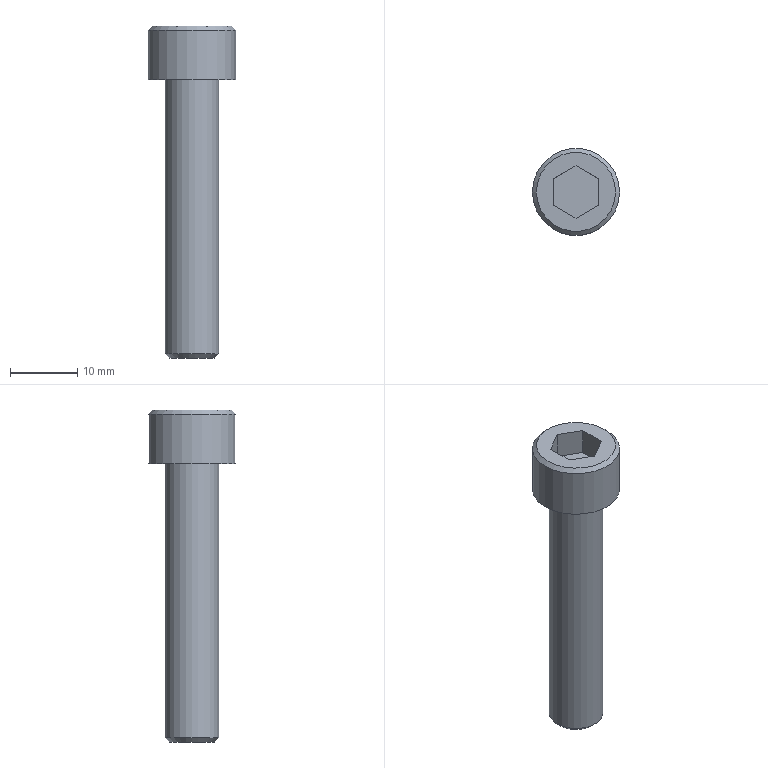Part | NX | features M8.00-50.00 2 | 1 solid | 14 faces | box 13 x 13 x 49.5 mm | volume 2976 mm3 | plane 10 | cylinder 2 | cone 2 | commonest cylinder face diameters 8 x1 13 x1
STEP:
#1=CARTESIAN_POINT('',(160.9,106.5,-1.5));
#2=VERTEX_POINT('',#1);
#3=CARTESIAN_POINT('',(155.,106.5,-1.5));
#4=DIRECTION('',(0.,0.,1.));
#5=DIRECTION('',(1.,0.,0.));
#6=AXIS2_PLACEMENT_3D('',#3,#4,#5);
#7=CIRCLE('',#6,5.9);
#8=EDGE_CURVE('',#2,#2,#7,.T.);
#9=ORIENTED_EDGE('',*,*,#8,.T.);
#10=EDGE_LOOP('',(#9));
#11=FACE_BOUND('',#10,.T.);
#12=CARTESIAN_POINT('',(151.6,108.463,-1.5));
#13=VERTEX_POINT('',#12);
#14=CARTESIAN_POINT('',(151.6,104.537,-1.5));
#15=VERTEX_POINT('',#14);
#16=CARTESIAN_POINT('',(151.6,108.463,-1.5));
#17=DIRECTION('',(0.,-1.,0.));
#18=VECTOR('',#17,1000.);
#19=LINE('',#16,#18);
#20=EDGE_CURVE('',#13,#15,#19,.T.);
#21=ORIENTED_EDGE('',*,*,#20,.F.);
#22=CARTESIAN_POINT('',(155.,110.426,-1.5));
#23=VERTEX_POINT('',#22);
#24=CARTESIAN_POINT('',(155.,110.426,-1.5));
#25=DIRECTION('',(-0.866,-0.5,0.));
#26=VECTOR('',#25,1000.);
#27=LINE('',#24,#26);
#28=EDGE_CURVE('',#23,#13,#27,.T.);
#29=ORIENTED_EDGE('',*,*,#28,.F.);
#30=CARTESIAN_POINT('',(158.4,108.463,-1.5));
#31=VERTEX_POINT('',#30);
#32=CARTESIAN_POINT('',(158.4,108.463,-1.5));
#33=DIRECTION('',(-0.866,0.5,0.));
#34=VECTOR('',#33,1000.);
#35=LINE('',#32,#34);
#36=EDGE_CURVE('',#31,#23,#35,.T.);
#37=ORIENTED_EDGE('',*,*,#36,.F.);
#38=CARTESIAN_POINT('',(158.4,104.537,-1.5));
#39=VERTEX_POINT('',#38);
#40=CARTESIAN_POINT('',(158.4,104.537,-1.5));
#41=DIRECTION('',(0.,1.,0.));
#42=VECTOR('',#41,1000.);
#43=LINE('',#40,#42);
#44=EDGE_CURVE('',#39,#31,#43,.T.);
#45=ORIENTED_EDGE('',*,*,#44,.F.);
#46=CARTESIAN_POINT('',(155.,102.574,-1.5));
#47=VERTEX_POINT('',#46);
#48=CARTESIAN_POINT('',(155.,102.574,-1.5));
#49=DIRECTION('',(0.866,0.5,0.));
#50=VECTOR('',#49,1000.);
#51=LINE('',#48,#50);
#52=EDGE_CURVE('',#47,#39,#51,.T.);
#53=ORIENTED_EDGE('',*,*,#52,.F.);
#54=CARTESIAN_POINT('',(151.6,104.537,-1.5));
#55=DIRECTION('',(0.866,-0.5,0.));
#56=VECTOR('',#55,1000.);
#57=LINE('',#54,#56);
#58=EDGE_CURVE('',#15,#47,#57,.T.);
#59=ORIENTED_EDGE('',*,*,#58,.F.);
#60=EDGE_LOOP('',(#21,#29,#37,#45,#53,#59));
#61=FACE_BOUND('',#60,.T.);
#62=CARTESIAN_POINT('',(155.,106.5,-1.5));
#63=DIRECTION('',(0.,0.,1.));
#64=DIRECTION('',(1.,0.,0.));
#65=AXIS2_PLACEMENT_3D('',#62,#63,#64);
#66=PLANE('',#65);
#67=ADVANCED_FACE('',(#11,#61),#66,.T.);
#68=CARTESIAN_POINT('',(159.,106.5,-9.5));
#69=VERTEX_POINT('',#68);
#70=CARTESIAN_POINT('',(155.,106.5,-9.5));
#71=DIRECTION('',(0.,0.,-1.));
#72=DIRECTION('',(1.,0.,0.));
#73=AXIS2_PLACEMENT_3D('',#70,#71,#72);
#74=CIRCLE('',#73,4.);
#75=EDGE_CURVE('',#69,#69,#74,.T.);
#76=ORIENTED_EDGE('',*,*,#75,.F.);
#77=EDGE_LOOP('',(#76));
#78=FACE_BOUND('',#77,.T.);
#79=CARTESIAN_POINT('',(161.5,106.5,-9.5));
#80=VERTEX_POINT('',#79);
#81=CARTESIAN_POINT('',(155.,106.5,-9.5));
#82=DIRECTION('',(0.,0.,1.));
#83=DIRECTION('',(1.,0.,0.));
#84=AXIS2_PLACEMENT_3D('',#81,#82,#83);
#85=CIRCLE('',#84,6.5);
#86=EDGE_CURVE('',#80,#80,#85,.T.);
#87=ORIENTED_EDGE('',*,*,#86,.F.);
#88=EDGE_LOOP('',(#87));
#89=FACE_BOUND('',#88,.T.);
#90=CARTESIAN_POINT('',(155.,106.5,-9.5));
#91=DIRECTION('',(0.,0.,-1.));
#92=DIRECTION('',(-1.,0.,0.));
#93=AXIS2_PLACEMENT_3D('',#90,#91,#92);
#94=PLANE('',#93);
#95=ADVANCED_FACE('',(#78,#89),#94,.T.);
#96=CARTESIAN_POINT('',(161.5,106.5,-2.1));
#97=VERTEX_POINT('',#96);
#98=CARTESIAN_POINT('',(155.,106.5,-2.1));
#99=DIRECTION('',(0.,0.,1.));
#100=DIRECTION('',(1.,0.,0.));
#101=AXIS2_PLACEMENT_3D('',#98,#99,#100);
#102=CIRCLE('',#101,6.5);
#103=EDGE_CURVE('',#97,#97,#102,.F.);
#104=ORIENTED_EDGE('',*,*,#103,.T.);
#105=EDGE_LOOP('',(#104));
#106=FACE_BOUND('',#105,.T.);
#107=ORIENTED_EDGE('',*,*,#86,.T.);
#108=EDGE_LOOP('',(#107));
#109=FACE_BOUND('',#108,.T.);
#110=CARTESIAN_POINT('',(155.,106.5,-9.5));
#111=DIRECTION('',(0.,0.,1.));
#112=DIRECTION('',(1.,0.,0.));
#113=AXIS2_PLACEMENT_3D('',#110,#111,#112);
#114=CYLINDRICAL_SURFACE('',#113,6.5);
#115=ADVANCED_FACE('',(#106,#109),#114,.T.);
#116=CARTESIAN_POINT('',(151.6,106.5,-51.));
#117=VERTEX_POINT('',#116);
#118=CARTESIAN_POINT('',(155.,106.5,-51.));
#119=DIRECTION('',(0.,0.,-1.));
#120=DIRECTION('',(-1.,0.,0.));
#121=AXIS2_PLACEMENT_3D('',#118,#119,#120);
#122=CIRCLE('',#121,3.4);
#123=EDGE_CURVE('',#117,#117,#122,.T.);
#124=ORIENTED_EDGE('',*,*,#123,.T.);
#125=EDGE_LOOP('',(#124));
#126=FACE_BOUND('',#125,.T.);
#127=CARTESIAN_POINT('',(155.,106.5,-51.));
#128=DIRECTION('',(0.,0.,-1.));
#129=DIRECTION('',(-1.,0.,0.));
#130=AXIS2_PLACEMENT_3D('',#127,#128,#129);
#131=PLANE('',#130);
#132=ADVANCED_FACE('',(#126),#131,.T.);
#133=CARTESIAN_POINT('',(151.,106.5,-50.4));
#134=VERTEX_POINT('',#133);
#135=CARTESIAN_POINT('',(155.,106.5,-50.4));
#136=DIRECTION('',(0.,0.,-1.));
#137=DIRECTION('',(-1.,0.,0.));
#138=AXIS2_PLACEMENT_3D('',#135,#136,#137);
#139=CIRCLE('',#138,4.);
#140=EDGE_CURVE('',#134,#134,#139,.F.);
#141=ORIENTED_EDGE('',*,*,#140,.T.);
#142=EDGE_LOOP('',(#141));
#143=FACE_BOUND('',#142,.T.);
#144=ORIENTED_EDGE('',*,*,#75,.T.);
#145=EDGE_LOOP('',(#144));
#146=FACE_BOUND('',#145,.T.);
#147=CARTESIAN_POINT('',(155.,106.5,-9.5));
#148=DIRECTION('',(0.,0.,-1.));
#149=DIRECTION('',(1.,0.,0.));
#150=AXIS2_PLACEMENT_3D('',#147,#148,#149);
#151=CYLINDRICAL_SURFACE('',#150,4.);
#152=ADVANCED_FACE('',(#143,#146),#151,.T.);
#153=ORIENTED_EDGE('',*,*,#58,.T.);
#154=CARTESIAN_POINT('',(155.,102.574,-5.5));
#155=VERTEX_POINT('',#154);
#156=CARTESIAN_POINT('',(155.,102.574,-5.5));
#157=DIRECTION('',(0.,0.,1.));
#158=VECTOR('',#157,1000.);
#159=LINE('',#156,#158);
#160=EDGE_CURVE('',#47,#155,#159,.F.);
#161=ORIENTED_EDGE('',*,*,#160,.T.);
#162=CARTESIAN_POINT('',(151.6,104.537,-5.5));
#163=VERTEX_POINT('',#162);
#164=CARTESIAN_POINT('',(151.6,104.537,-5.5));
#165=DIRECTION('',(0.866,-0.5,0.));
#166=VECTOR('',#165,1000.);
#167=LINE('',#164,#166);
#168=EDGE_CURVE('',#155,#163,#167,.F.);
#169=ORIENTED_EDGE('',*,*,#168,.T.);
#170=CARTESIAN_POINT('',(151.6,104.537,-5.5));
#171=DIRECTION('',(0.,0.,1.));
#172=VECTOR('',#171,1000.);
#173=LINE('',#170,#172);
#174=EDGE_CURVE('',#15,#163,#173,.F.);
#175=ORIENTED_EDGE('',*,*,#174,.F.);
#176=EDGE_LOOP('',(#153,#161,#169,#175));
#177=FACE_BOUND('',#176,.T.);
#178=CARTESIAN_POINT('',(153.3,103.556,-3.5));
#179=DIRECTION('',(-0.5,-0.866,0.));
#180=DIRECTION('',(0.866,-0.5,0.));
#181=AXIS2_PLACEMENT_3D('',#178,#179,#180);
#182=PLANE('',#181);
#183=ADVANCED_FACE('',(#177),#182,.F.);
#184=ORIENTED_EDGE('',*,*,#20,.T.);
#185=ORIENTED_EDGE('',*,*,#174,.T.);
#186=CARTESIAN_POINT('',(151.6,108.463,-5.5));
#187=VERTEX_POINT('',#186);
#188=CARTESIAN_POINT('',(151.6,108.463,-5.5));
#189=DIRECTION('',(0.,-1.,0.));
#190=VECTOR('',#189,1000.);
#191=LINE('',#188,#190);
#192=EDGE_CURVE('',#163,#187,#191,.F.);
#193=ORIENTED_EDGE('',*,*,#192,.T.);
#194=CARTESIAN_POINT('',(151.6,108.463,-5.5));
#195=DIRECTION('',(0.,0.,1.));
#196=VECTOR('',#195,1000.);
#197=LINE('',#194,#196);
#198=EDGE_CURVE('',#13,#187,#197,.F.);
#199=ORIENTED_EDGE('',*,*,#198,.F.);
#200=EDGE_LOOP('',(#184,#185,#193,#199));
#201=FACE_BOUND('',#200,.T.);
#202=CARTESIAN_POINT('',(151.6,106.5,-3.5));
#203=DIRECTION('',(-1.,0.,0.));
#204=DIRECTION('',(0.,0.,1.));
#205=AXIS2_PLACEMENT_3D('',#202,#203,#204);
#206=PLANE('',#205);
#207=ADVANCED_FACE('',(#201),#206,.F.);
#208=ORIENTED_EDGE('',*,*,#28,.T.);
#209=ORIENTED_EDGE('',*,*,#198,.T.);
#210=CARTESIAN_POINT('',(155.,110.426,-5.5));
#211=VERTEX_POINT('',#210);
#212=CARTESIAN_POINT('',(155.,110.426,-5.5));
#213=DIRECTION('',(-0.866,-0.5,0.));
#214=VECTOR('',#213,1000.);
#215=LINE('',#212,#214);
#216=EDGE_CURVE('',#187,#211,#215,.F.);
#217=ORIENTED_EDGE('',*,*,#216,.T.);
#218=CARTESIAN_POINT('',(155.,110.426,-5.5));
#219=DIRECTION('',(0.,0.,1.));
#220=VECTOR('',#219,1000.);
#221=LINE('',#218,#220);
#222=EDGE_CURVE('',#23,#211,#221,.F.);
#223=ORIENTED_EDGE('',*,*,#222,.F.);
#224=EDGE_LOOP('',(#208,#209,#217,#223));
#225=FACE_BOUND('',#224,.T.);
#226=CARTESIAN_POINT('',(153.3,109.444,-3.5));
#227=DIRECTION('',(-0.5,0.866,0.));
#228=DIRECTION('',(-0.866,-0.5,0.));
#229=AXIS2_PLACEMENT_3D('',#226,#227,#228);
#230=PLANE('',#229);
#231=ADVANCED_FACE('',(#225),#230,.F.);
#232=ORIENTED_EDGE('',*,*,#36,.T.);
#233=ORIENTED_EDGE('',*,*,#222,.T.);
#234=CARTESIAN_POINT('',(158.4,108.463,-5.5));
#235=VERTEX_POINT('',#234);
#236=CARTESIAN_POINT('',(158.4,108.463,-5.5));
#237=DIRECTION('',(-0.866,0.5,0.));
#238=VECTOR('',#237,1000.);
#239=LINE('',#236,#238);
#240=EDGE_CURVE('',#211,#235,#239,.F.);
#241=ORIENTED_EDGE('',*,*,#240,.T.);
#242=CARTESIAN_POINT('',(158.4,108.463,-5.5));
#243=DIRECTION('',(0.,0.,1.));
#244=VECTOR('',#243,1000.);
#245=LINE('',#242,#244);
#246=EDGE_CURVE('',#31,#235,#245,.F.);
#247=ORIENTED_EDGE('',*,*,#246,.F.);
#248=EDGE_LOOP('',(#232,#233,#241,#247));
#249=FACE_BOUND('',#248,.T.);
#250=CARTESIAN_POINT('',(156.7,109.444,-3.5));
#251=DIRECTION('',(0.5,0.866,0.));
#252=DIRECTION('',(-0.866,0.5,0.));
#253=AXIS2_PLACEMENT_3D('',#250,#251,#252);
#254=PLANE('',#253);
#255=ADVANCED_FACE('',(#249),#254,.F.);
#256=ORIENTED_EDGE('',*,*,#44,.T.);
#257=ORIENTED_EDGE('',*,*,#246,.T.);
#258=CARTESIAN_POINT('',(158.4,104.537,-5.5));
#259=VERTEX_POINT('',#258);
#260=CARTESIAN_POINT('',(158.4,104.537,-5.5));
#261=DIRECTION('',(0.,1.,0.));
#262=VECTOR('',#261,1000.);
#263=LINE('',#260,#262);
#264=EDGE_CURVE('',#235,#259,#263,.F.);
#265=ORIENTED_EDGE('',*,*,#264,.T.);
#266=CARTESIAN_POINT('',(158.4,104.537,-5.5));
#267=DIRECTION('',(0.,0.,1.));
#268=VECTOR('',#267,1000.);
#269=LINE('',#266,#268);
#270=EDGE_CURVE('',#39,#259,#269,.F.);
#271=ORIENTED_EDGE('',*,*,#270,.F.);
#272=EDGE_LOOP('',(#256,#257,#265,#271));
#273=FACE_BOUND('',#272,.T.);
#274=CARTESIAN_POINT('',(158.4,106.5,-3.5));
#275=DIRECTION('',(1.,0.,0.));
#276=DIRECTION('',(0.,0.,-1.));
#277=AXIS2_PLACEMENT_3D('',#274,#275,#276);
#278=PLANE('',#277);
#279=ADVANCED_FACE('',(#273),#278,.F.);
#280=ORIENTED_EDGE('',*,*,#52,.T.);
#281=ORIENTED_EDGE('',*,*,#270,.T.);
#282=CARTESIAN_POINT('',(155.,102.574,-5.5));
#283=DIRECTION('',(0.866,0.5,0.));
#284=VECTOR('',#283,1000.);
#285=LINE('',#282,#284);
#286=EDGE_CURVE('',#259,#155,#285,.F.);
#287=ORIENTED_EDGE('',*,*,#286,.T.);
#288=ORIENTED_EDGE('',*,*,#160,.F.);
#289=EDGE_LOOP('',(#280,#281,#287,#288));
#290=FACE_BOUND('',#289,.T.);
#291=CARTESIAN_POINT('',(156.7,103.556,-3.5));
#292=DIRECTION('',(0.5,-0.866,0.));
#293=DIRECTION('',(0.866,0.5,0.));
#294=AXIS2_PLACEMENT_3D('',#291,#292,#293);
#295=PLANE('',#294);
#296=ADVANCED_FACE('',(#290),#295,.F.);
#297=ORIENTED_EDGE('',*,*,#286,.F.);
#298=ORIENTED_EDGE('',*,*,#264,.F.);
#299=ORIENTED_EDGE('',*,*,#240,.F.);
#300=ORIENTED_EDGE('',*,*,#216,.F.);
#301=ORIENTED_EDGE('',*,*,#192,.F.);
#302=ORIENTED_EDGE('',*,*,#168,.F.);
#303=EDGE_LOOP('',(#297,#298,#299,#300,#301,#302));
#304=FACE_BOUND('',#303,.T.);
#305=CARTESIAN_POINT('',(155.,106.5,-5.5));
#306=DIRECTION('',(0.,0.,-1.));
#307=DIRECTION('',(-1.,0.,0.));
#308=AXIS2_PLACEMENT_3D('',#305,#306,#307);
#309=PLANE('',#308);
#310=ADVANCED_FACE('',(#304),#309,.F.);
#311=ORIENTED_EDGE('',*,*,#123,.F.);
#312=EDGE_LOOP('',(#311));
#313=FACE_BOUND('',#312,.T.);
#314=ORIENTED_EDGE('',*,*,#140,.F.);
#315=EDGE_LOOP('',(#314));
#316=FACE_BOUND('',#315,.T.);
#317=CARTESIAN_POINT('',(155.,106.5,-50.4));
#318=DIRECTION('',(0.,0.,1.));
#319=DIRECTION('',(1.,0.,0.));
#320=AXIS2_PLACEMENT_3D('',#317,#318,#319);
#321=CONICAL_SURFACE('',#320,4.,0.7854);
#322=ADVANCED_FACE('',(#313,#316),#321,.T.);
#323=ORIENTED_EDGE('',*,*,#8,.F.);
#324=EDGE_LOOP('',(#323));
#325=FACE_BOUND('',#324,.T.);
#326=ORIENTED_EDGE('',*,*,#103,.F.);
#327=EDGE_LOOP('',(#326));
#328=FACE_BOUND('',#327,.T.);
#329=CARTESIAN_POINT('',(155.,106.5,-2.1));
#330=DIRECTION('',(0.,0.,-1.));
#331=DIRECTION('',(-1.,0.,0.));
#332=AXIS2_PLACEMENT_3D('',#329,#330,#331);
#333=CONICAL_SURFACE('',#332,6.5,0.7854);
#334=ADVANCED_FACE('',(#325,#328),#333,.T.);
#335=CLOSED_SHELL('',(#67,#95,#115,#132,#152,#183,#207,#231,#255,#279,#296,#310,#322,#334));
#336=MANIFOLD_SOLID_BREP('',#335);
#337=(LENGTH_UNIT()NAMED_UNIT(*)SI_UNIT(.MILLI.,.METRE.));
#338=UNCERTAINTY_MEASURE_WITH_UNIT(LENGTH_MEASURE(0.00001),#337,'','');
#339=(NAMED_UNIT(*)PLANE_ANGLE_UNIT()SI_UNIT($,.RADIAN.));
#340=(NAMED_UNIT(*)SI_UNIT($,.STERADIAN.)SOLID_ANGLE_UNIT());
#341=(GEOMETRIC_REPRESENTATION_CONTEXT(3)GLOBAL_UNCERTAINTY_ASSIGNED_CONTEXT((#338))GLOBAL_UNIT_ASSIGNED_CONTEXT((#337,#339,#340))REPRESENTATION_CONTEXT('',''));
#342=ADVANCED_BREP_SHAPE_REPRESENTATION('',(#336),#341);